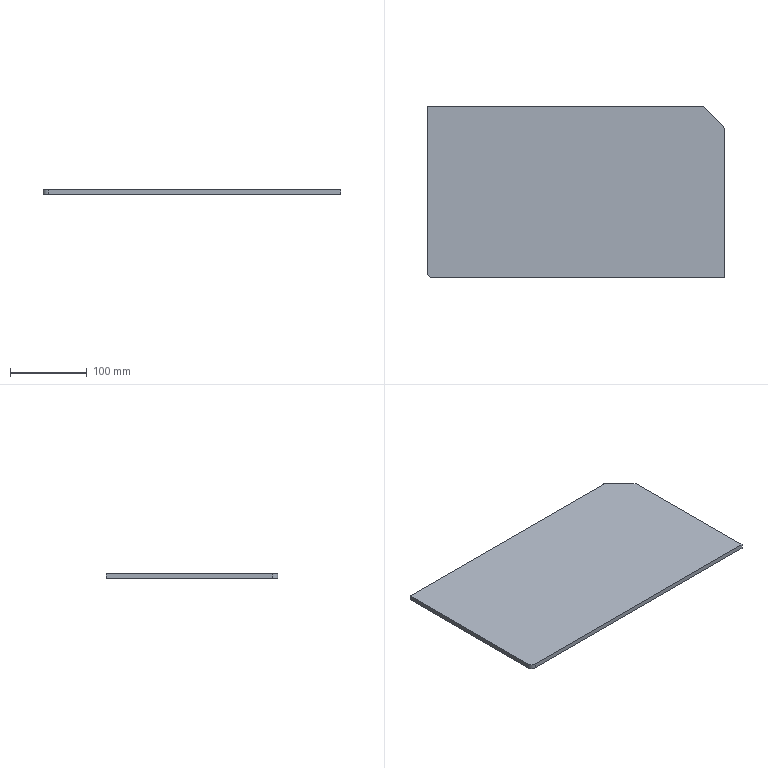Part | SolidWorks | features FlatPattern 1, SMBaseFlange 1, SheetMetal 1 | 1 solid | 10 faces | box 388 x 224 x 6 mm | volume 518873 mm3 | plane 7 | cylinder 3 | commonest cylinder face diameters 14 x3
STEP:
#1=CARTESIAN_POINT('',(388.,0.,0.));
#2=VERTEX_POINT('',#1);
#3=CARTESIAN_POINT('',(388.,192.101,0.));
#4=VERTEX_POINT('',#3);
#5=CARTESIAN_POINT('',(388.,0.,0.));
#6=DIRECTION('',(0.,1.,0.));
#7=VECTOR('',#6,1000.);
#8=LINE('',#5,#7);
#9=EDGE_CURVE('',#2,#4,#8,.T.);
#10=ORIENTED_EDGE('',*,*,#9,.F.);
#11=CARTESIAN_POINT('',(388.,0.,-6.));
#12=VERTEX_POINT('',#11);
#13=CARTESIAN_POINT('',(388.,0.,-6.));
#14=DIRECTION('',(0.,0.,1.));
#15=VECTOR('',#14,1000.);
#16=LINE('',#13,#15);
#17=EDGE_CURVE('',#12,#2,#16,.T.);
#18=ORIENTED_EDGE('',*,*,#17,.F.);
#19=CARTESIAN_POINT('',(388.,192.101,-6.));
#20=VERTEX_POINT('',#19);
#21=CARTESIAN_POINT('',(388.,0.,-6.));
#22=DIRECTION('',(0.,1.,0.));
#23=VECTOR('',#22,1000.);
#24=LINE('',#21,#23);
#25=EDGE_CURVE('',#12,#20,#24,.T.);
#26=ORIENTED_EDGE('',*,*,#25,.T.);
#27=CARTESIAN_POINT('',(388.,192.101,-6.));
#28=DIRECTION('',(0.,0.,1.));
#29=VECTOR('',#28,1000.);
#30=LINE('',#27,#29);
#31=EDGE_CURVE('',#20,#4,#30,.T.);
#32=ORIENTED_EDGE('',*,*,#31,.T.);
#33=EDGE_LOOP('',(#10,#18,#26,#32));
#34=FACE_OUTER_BOUND('',#33,.T.);
#35=CARTESIAN_POINT('',(388.,0.,-6.));
#36=DIRECTION('',(1.,0.,0.));
#37=DIRECTION('',(0.,0.,-1.));
#38=AXIS2_PLACEMENT_3D('',#35,#36,#37);
#39=PLANE('',#38);
#40=ADVANCED_FACE('',(#34),#39,.T.);
#41=CARTESIAN_POINT('',(7.,0.,0.));
#42=VERTEX_POINT('',#41);
#43=CARTESIAN_POINT('',(7.,0.,0.));
#44=DIRECTION('',(1.,0.,0.));
#45=VECTOR('',#44,1000.);
#46=LINE('',#43,#45);
#47=EDGE_CURVE('',#42,#2,#46,.T.);
#48=ORIENTED_EDGE('',*,*,#47,.F.);
#49=CARTESIAN_POINT('',(7.,0.,-6.));
#50=VERTEX_POINT('',#49);
#51=CARTESIAN_POINT('',(7.,0.,-6.));
#52=DIRECTION('',(0.,0.,1.));
#53=VECTOR('',#52,1000.);
#54=LINE('',#51,#53);
#55=EDGE_CURVE('',#50,#42,#54,.T.);
#56=ORIENTED_EDGE('',*,*,#55,.F.);
#57=CARTESIAN_POINT('',(7.,0.,-6.));
#58=DIRECTION('',(1.,0.,0.));
#59=VECTOR('',#58,1000.);
#60=LINE('',#57,#59);
#61=EDGE_CURVE('',#50,#12,#60,.T.);
#62=ORIENTED_EDGE('',*,*,#61,.T.);
#63=ORIENTED_EDGE('',*,*,#17,.T.);
#64=EDGE_LOOP('',(#48,#56,#62,#63));
#65=FACE_OUTER_BOUND('',#64,.T.);
#66=CARTESIAN_POINT('',(7.,0.,-6.));
#67=DIRECTION('',(0.,-1.,0.));
#68=DIRECTION('',(0.,0.,-1.));
#69=AXIS2_PLACEMENT_3D('',#66,#67,#68);
#70=PLANE('',#69);
#71=ADVANCED_FACE('',(#65),#70,.T.);
#72=CARTESIAN_POINT('',(0.,7.,0.));
#73=VERTEX_POINT('',#72);
#74=CARTESIAN_POINT('',(7.,7.,0.));
#75=DIRECTION('',(0.,0.,1.));
#76=DIRECTION('',(-1.,0.,0.));
#77=AXIS2_PLACEMENT_3D('',#74,#75,#76);
#78=CIRCLE('',#77,7.);
#79=EDGE_CURVE('',#73,#42,#78,.T.);
#80=ORIENTED_EDGE('',*,*,#79,.F.);
#81=CARTESIAN_POINT('',(0.,7.,-6.));
#82=VERTEX_POINT('',#81);
#83=CARTESIAN_POINT('',(0.,7.,-6.));
#84=DIRECTION('',(0.,0.,1.));
#85=VECTOR('',#84,1000.);
#86=LINE('',#83,#85);
#87=EDGE_CURVE('',#82,#73,#86,.T.);
#88=ORIENTED_EDGE('',*,*,#87,.F.);
#89=CARTESIAN_POINT('',(7.,7.,-6.));
#90=DIRECTION('',(0.,0.,1.));
#91=DIRECTION('',(-1.,0.,0.));
#92=AXIS2_PLACEMENT_3D('',#89,#90,#91);
#93=CIRCLE('',#92,7.);
#94=EDGE_CURVE('',#82,#50,#93,.T.);
#95=ORIENTED_EDGE('',*,*,#94,.T.);
#96=ORIENTED_EDGE('',*,*,#55,.T.);
#97=EDGE_LOOP('',(#80,#88,#95,#96));
#98=FACE_OUTER_BOUND('',#97,.T.);
#99=CARTESIAN_POINT('',(7.,7.,-6.));
#100=DIRECTION('',(0.,0.,1.));
#101=DIRECTION('',(1.,0.,0.));
#102=AXIS2_PLACEMENT_3D('',#99,#100,#101);
#103=CYLINDRICAL_SURFACE('',#102,7.);
#104=ADVANCED_FACE('',(#98),#103,.T.);
#105=CARTESIAN_POINT('',(0.,224.,0.));
#106=VERTEX_POINT('',#105);
#107=CARTESIAN_POINT('',(0.,224.,0.));
#108=DIRECTION('',(0.,-1.,0.));
#109=VECTOR('',#108,1000.);
#110=LINE('',#107,#109);
#111=EDGE_CURVE('',#106,#73,#110,.T.);
#112=ORIENTED_EDGE('',*,*,#111,.F.);
#113=CARTESIAN_POINT('',(0.,224.,-6.));
#114=VERTEX_POINT('',#113);
#115=CARTESIAN_POINT('',(0.,224.,-6.));
#116=DIRECTION('',(0.,0.,1.));
#117=VECTOR('',#116,1000.);
#118=LINE('',#115,#117);
#119=EDGE_CURVE('',#114,#106,#118,.T.);
#120=ORIENTED_EDGE('',*,*,#119,.F.);
#121=CARTESIAN_POINT('',(0.,224.,-6.));
#122=DIRECTION('',(0.,-1.,0.));
#123=VECTOR('',#122,1000.);
#124=LINE('',#121,#123);
#125=EDGE_CURVE('',#114,#82,#124,.T.);
#126=ORIENTED_EDGE('',*,*,#125,.T.);
#127=ORIENTED_EDGE('',*,*,#87,.T.);
#128=EDGE_LOOP('',(#112,#120,#126,#127));
#129=FACE_OUTER_BOUND('',#128,.T.);
#130=CARTESIAN_POINT('',(0.,224.,-6.));
#131=DIRECTION('',(-1.,0.,0.));
#132=DIRECTION('',(0.,-1.,0.));
#133=AXIS2_PLACEMENT_3D('',#130,#131,#132);
#134=PLANE('',#133);
#135=ADVANCED_FACE('',(#129),#134,.T.);
#136=CARTESIAN_POINT('',(356.101,224.,0.));
#137=VERTEX_POINT('',#136);
#138=CARTESIAN_POINT('',(356.101,224.,0.));
#139=DIRECTION('',(-1.,0.,0.));
#140=VECTOR('',#139,1000.);
#141=LINE('',#138,#140);
#142=EDGE_CURVE('',#137,#106,#141,.T.);
#143=ORIENTED_EDGE('',*,*,#142,.F.);
#144=CARTESIAN_POINT('',(356.101,224.,-6.));
#145=VERTEX_POINT('',#144);
#146=CARTESIAN_POINT('',(356.101,224.,-6.));
#147=DIRECTION('',(0.,0.,1.));
#148=VECTOR('',#147,1000.);
#149=LINE('',#146,#148);
#150=EDGE_CURVE('',#145,#137,#149,.T.);
#151=ORIENTED_EDGE('',*,*,#150,.F.);
#152=CARTESIAN_POINT('',(356.101,224.,-6.));
#153=DIRECTION('',(-1.,0.,0.));
#154=VECTOR('',#153,1000.);
#155=LINE('',#152,#154);
#156=EDGE_CURVE('',#145,#114,#155,.T.);
#157=ORIENTED_EDGE('',*,*,#156,.T.);
#158=ORIENTED_EDGE('',*,*,#119,.T.);
#159=EDGE_LOOP('',(#143,#151,#157,#158));
#160=FACE_OUTER_BOUND('',#159,.T.);
#161=CARTESIAN_POINT('',(356.101,224.,-6.));
#162=DIRECTION('',(0.,1.,0.));
#163=DIRECTION('',(-1.,0.,0.));
#164=AXIS2_PLACEMENT_3D('',#161,#162,#163);
#165=PLANE('',#164);
#166=ADVANCED_FACE('',(#160),#165,.T.);
#167=CARTESIAN_POINT('',(361.05,221.95,0.));
#168=VERTEX_POINT('',#167);
#169=CARTESIAN_POINT('',(356.101,217.,0.));
#170=DIRECTION('',(0.,0.,1.));
#171=DIRECTION('',(1.,0.,0.));
#172=AXIS2_PLACEMENT_3D('',#169,#170,#171);
#173=CIRCLE('',#172,7.);
#174=EDGE_CURVE('',#168,#137,#173,.T.);
#175=ORIENTED_EDGE('',*,*,#174,.F.);
#176=CARTESIAN_POINT('',(361.05,221.95,-6.));
#177=VERTEX_POINT('',#176);
#178=CARTESIAN_POINT('',(361.05,221.95,-6.));
#179=DIRECTION('',(0.,0.,1.));
#180=VECTOR('',#179,1000.);
#181=LINE('',#178,#180);
#182=EDGE_CURVE('',#177,#168,#181,.T.);
#183=ORIENTED_EDGE('',*,*,#182,.F.);
#184=CARTESIAN_POINT('',(356.101,217.,-6.));
#185=DIRECTION('',(0.,0.,1.));
#186=DIRECTION('',(1.,0.,0.));
#187=AXIS2_PLACEMENT_3D('',#184,#185,#186);
#188=CIRCLE('',#187,7.);
#189=EDGE_CURVE('',#177,#145,#188,.T.);
#190=ORIENTED_EDGE('',*,*,#189,.T.);
#191=ORIENTED_EDGE('',*,*,#150,.T.);
#192=EDGE_LOOP('',(#175,#183,#190,#191));
#193=FACE_OUTER_BOUND('',#192,.T.);
#194=CARTESIAN_POINT('',(356.101,217.,-6.));
#195=DIRECTION('',(0.,0.,1.));
#196=DIRECTION('',(1.,0.,0.));
#197=AXIS2_PLACEMENT_3D('',#194,#195,#196);
#198=CYLINDRICAL_SURFACE('',#197,7.);
#199=ADVANCED_FACE('',(#193),#198,.T.);
#200=CARTESIAN_POINT('',(385.95,197.05,0.));
#201=VERTEX_POINT('',#200);
#202=CARTESIAN_POINT('',(385.95,197.05,0.));
#203=DIRECTION('',(-0.7071,0.7071,0.));
#204=VECTOR('',#203,1000.);
#205=LINE('',#202,#204);
#206=EDGE_CURVE('',#201,#168,#205,.T.);
#207=ORIENTED_EDGE('',*,*,#206,.F.);
#208=CARTESIAN_POINT('',(385.95,197.05,-6.));
#209=VERTEX_POINT('',#208);
#210=CARTESIAN_POINT('',(385.95,197.05,-6.));
#211=DIRECTION('',(0.,0.,1.));
#212=VECTOR('',#211,1000.);
#213=LINE('',#210,#212);
#214=EDGE_CURVE('',#209,#201,#213,.T.);
#215=ORIENTED_EDGE('',*,*,#214,.F.);
#216=CARTESIAN_POINT('',(385.95,197.05,-6.));
#217=DIRECTION('',(-0.7071,0.7071,0.));
#218=VECTOR('',#217,1000.);
#219=LINE('',#216,#218);
#220=EDGE_CURVE('',#209,#177,#219,.T.);
#221=ORIENTED_EDGE('',*,*,#220,.T.);
#222=ORIENTED_EDGE('',*,*,#182,.T.);
#223=EDGE_LOOP('',(#207,#215,#221,#222));
#224=FACE_OUTER_BOUND('',#223,.T.);
#225=CARTESIAN_POINT('',(385.95,197.05,-6.));
#226=DIRECTION('',(0.7071,0.7071,0.));
#227=DIRECTION('',(-0.7071,0.7071,0.));
#228=AXIS2_PLACEMENT_3D('',#225,#226,#227);
#229=PLANE('',#228);
#230=ADVANCED_FACE('',(#224),#229,.T.);
#231=CARTESIAN_POINT('',(381.,192.101,0.));
#232=DIRECTION('',(0.,0.,1.));
#233=DIRECTION('',(1.,0.,0.));
#234=AXIS2_PLACEMENT_3D('',#231,#232,#233);
#235=CIRCLE('',#234,7.);
#236=EDGE_CURVE('',#4,#201,#235,.T.);
#237=ORIENTED_EDGE('',*,*,#236,.F.);
#238=ORIENTED_EDGE('',*,*,#31,.F.);
#239=CARTESIAN_POINT('',(381.,192.101,-6.));
#240=DIRECTION('',(0.,0.,1.));
#241=DIRECTION('',(1.,0.,0.));
#242=AXIS2_PLACEMENT_3D('',#239,#240,#241);
#243=CIRCLE('',#242,7.);
#244=EDGE_CURVE('',#20,#209,#243,.T.);
#245=ORIENTED_EDGE('',*,*,#244,.T.);
#246=ORIENTED_EDGE('',*,*,#214,.T.);
#247=EDGE_LOOP('',(#237,#238,#245,#246));
#248=FACE_OUTER_BOUND('',#247,.T.);
#249=CARTESIAN_POINT('',(381.,192.101,-6.));
#250=DIRECTION('',(0.,0.,1.));
#251=DIRECTION('',(1.,0.,0.));
#252=AXIS2_PLACEMENT_3D('',#249,#250,#251);
#253=CYLINDRICAL_SURFACE('',#252,7.);
#254=ADVANCED_FACE('',(#248),#253,.T.);
#255=ORIENTED_EDGE('',*,*,#25,.F.);
#256=ORIENTED_EDGE('',*,*,#61,.F.);
#257=ORIENTED_EDGE('',*,*,#94,.F.);
#258=ORIENTED_EDGE('',*,*,#125,.F.);
#259=ORIENTED_EDGE('',*,*,#156,.F.);
#260=ORIENTED_EDGE('',*,*,#189,.F.);
#261=ORIENTED_EDGE('',*,*,#220,.F.);
#262=ORIENTED_EDGE('',*,*,#244,.F.);
#263=EDGE_LOOP('',(#255,#256,#257,#258,#259,#260,#261,#262));
#264=FACE_OUTER_BOUND('',#263,.T.);
#265=CARTESIAN_POINT('',(381.,192.101,-6.));
#266=DIRECTION('',(0.,0.,1.));
#267=DIRECTION('',(1.,0.,0.));
#268=AXIS2_PLACEMENT_3D('',#265,#266,#267);
#269=PLANE('',#268);
#270=ADVANCED_FACE('',(#264),#269,.F.);
#271=ORIENTED_EDGE('',*,*,#9,.T.);
#272=ORIENTED_EDGE('',*,*,#236,.T.);
#273=ORIENTED_EDGE('',*,*,#206,.T.);
#274=ORIENTED_EDGE('',*,*,#174,.T.);
#275=ORIENTED_EDGE('',*,*,#142,.T.);
#276=ORIENTED_EDGE('',*,*,#111,.T.);
#277=ORIENTED_EDGE('',*,*,#79,.T.);
#278=ORIENTED_EDGE('',*,*,#47,.T.);
#279=EDGE_LOOP('',(#271,#272,#273,#274,#275,#276,#277,#278));
#280=FACE_OUTER_BOUND('',#279,.T.);
#281=CARTESIAN_POINT('',(381.,192.101,0.));
#282=DIRECTION('',(0.,0.,1.));
#283=DIRECTION('',(1.,0.,0.));
#284=AXIS2_PLACEMENT_3D('',#281,#282,#283);
#285=PLANE('',#284);
#286=ADVANCED_FACE('',(#280),#285,.T.);
#287=CLOSED_SHELL('',(#40,#71,#104,#135,#166,#199,#230,#254,#270,#286));
#288=MANIFOLD_SOLID_BREP('',#287);
#289=CARTESIAN_POINT('',(0.,0.,0.));
#290=DIRECTION('',(0.,0.,1.));
#291=DIRECTION('',(1.,0.,0.));
#292=AXIS2_PLACEMENT_3D('',#289,#290,#291);
#293=(LENGTH_UNIT()NAMED_UNIT(*)SI_UNIT(.MILLI.,.METRE.));
#294=UNCERTAINTY_MEASURE_WITH_UNIT(LENGTH_MEASURE(0.00001),#293,'','');
#295=(NAMED_UNIT(*)PLANE_ANGLE_UNIT()SI_UNIT($,.RADIAN.));
#296=(NAMED_UNIT(*)SI_UNIT($,.STERADIAN.)SOLID_ANGLE_UNIT());
#297=(GEOMETRIC_REPRESENTATION_CONTEXT(3)GLOBAL_UNCERTAINTY_ASSIGNED_CONTEXT((#294))GLOBAL_UNIT_ASSIGNED_CONTEXT((#293,#295,#296))REPRESENTATION_CONTEXT('',''));
#298=ADVANCED_BREP_SHAPE_REPRESENTATION('',(#288,#292),#297);